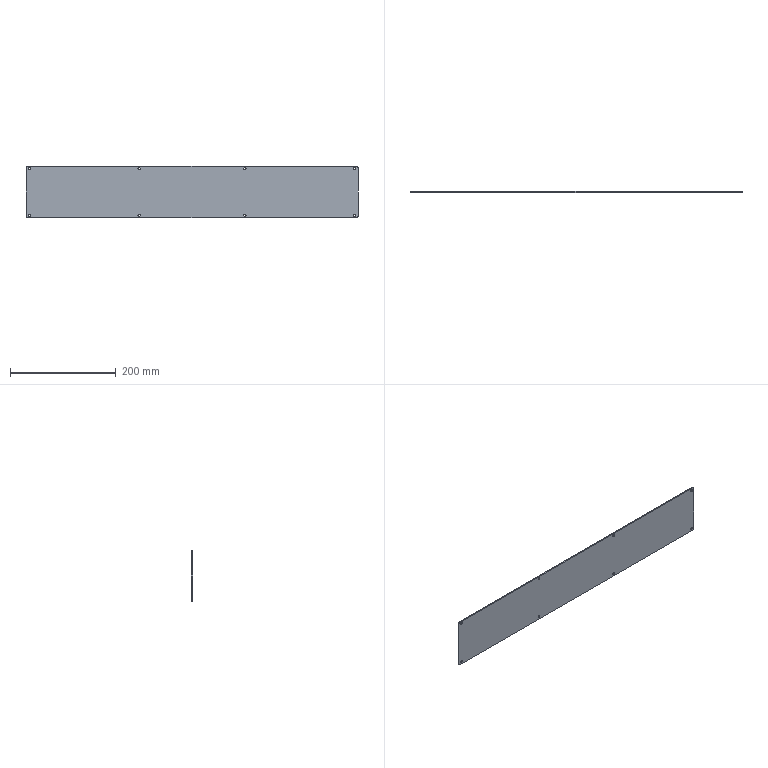Part | SolidWorks | features BaseBody 1 | 1 solid | 26 faces | box 628 x 2 x 98 mm | volume 122818 mm3 | cylinder 20 | plane 6 | commonest cylinder face diameters 4.5 x16 6 x4
STEP:
#1=CARTESIAN_POINT('',(307.5,0.,41.75));
#2=VERTEX_POINT('',#1);
#3=CARTESIAN_POINT('',(307.5,2.,41.75));
#4=VERTEX_POINT('',#3);
#5=CARTESIAN_POINT('',(307.5,-0.001,41.75));
#6=DIRECTION('',(0.,1.,0.));
#7=VECTOR('',#6,1000.);
#8=LINE('',#5,#7);
#9=EDGE_CURVE('',#2,#4,#8,.T.);
#10=ORIENTED_EDGE('',*,*,#9,.F.);
#11=CARTESIAN_POINT('',(307.5,0.,46.25));
#12=VERTEX_POINT('',#11);
#13=CARTESIAN_POINT('',(307.5,0.,44.));
#14=DIRECTION('',(0.,-1.,0.));
#15=DIRECTION('',(0.,0.,1.));
#16=AXIS2_PLACEMENT_3D('',#13,#14,#15);
#17=CIRCLE('',#16,2.25);
#18=EDGE_CURVE('',#2,#12,#17,.T.);
#19=ORIENTED_EDGE('',*,*,#18,.T.);
#20=CARTESIAN_POINT('',(307.5,2.,46.25));
#21=VERTEX_POINT('',#20);
#22=CARTESIAN_POINT('',(307.5,-0.001,46.25));
#23=DIRECTION('',(0.,1.,0.));
#24=VECTOR('',#23,1000.);
#25=LINE('',#22,#24);
#26=EDGE_CURVE('',#12,#21,#25,.T.);
#27=ORIENTED_EDGE('',*,*,#26,.T.);
#28=CARTESIAN_POINT('',(307.5,2.,44.));
#29=DIRECTION('',(0.,1.,0.));
#30=DIRECTION('',(0.,0.,1.));
#31=AXIS2_PLACEMENT_3D('',#28,#29,#30);
#32=CIRCLE('',#31,2.25);
#33=EDGE_CURVE('',#21,#4,#32,.T.);
#34=ORIENTED_EDGE('',*,*,#33,.T.);
#35=EDGE_LOOP('',(#10,#19,#27,#34));
#36=FACE_OUTER_BOUND('',#35,.T.);
#37=CARTESIAN_POINT('',(307.5,-0.001,44.));
#38=DIRECTION('',(0.,1.,0.));
#39=DIRECTION('',(0.,0.,1.));
#40=AXIS2_PLACEMENT_3D('',#37,#38,#39);
#41=CYLINDRICAL_SURFACE('',#40,2.25);
#42=ADVANCED_FACE('',(#36),#41,.F.);
#43=CARTESIAN_POINT('',(-307.5,0.,41.75));
#44=VERTEX_POINT('',#43);
#45=CARTESIAN_POINT('',(-307.5,2.,41.75));
#46=VERTEX_POINT('',#45);
#47=CARTESIAN_POINT('',(-307.5,-0.001,41.75));
#48=DIRECTION('',(0.,1.,0.));
#49=VECTOR('',#48,1000.);
#50=LINE('',#47,#49);
#51=EDGE_CURVE('',#44,#46,#50,.T.);
#52=ORIENTED_EDGE('',*,*,#51,.F.);
#53=CARTESIAN_POINT('',(-307.5,0.,46.25));
#54=VERTEX_POINT('',#53);
#55=CARTESIAN_POINT('',(-307.5,0.,44.));
#56=DIRECTION('',(0.,-1.,0.));
#57=DIRECTION('',(0.,0.,1.));
#58=AXIS2_PLACEMENT_3D('',#55,#56,#57);
#59=CIRCLE('',#58,2.25);
#60=EDGE_CURVE('',#44,#54,#59,.T.);
#61=ORIENTED_EDGE('',*,*,#60,.T.);
#62=CARTESIAN_POINT('',(-307.5,2.,46.25));
#63=VERTEX_POINT('',#62);
#64=CARTESIAN_POINT('',(-307.5,-0.001,46.25));
#65=DIRECTION('',(0.,1.,0.));
#66=VECTOR('',#65,1000.);
#67=LINE('',#64,#66);
#68=EDGE_CURVE('',#54,#63,#67,.T.);
#69=ORIENTED_EDGE('',*,*,#68,.T.);
#70=CARTESIAN_POINT('',(-307.5,2.,44.));
#71=DIRECTION('',(0.,1.,0.));
#72=DIRECTION('',(0.,0.,-1.));
#73=AXIS2_PLACEMENT_3D('',#70,#71,#72);
#74=CIRCLE('',#73,2.25);
#75=EDGE_CURVE('',#63,#46,#74,.T.);
#76=ORIENTED_EDGE('',*,*,#75,.T.);
#77=EDGE_LOOP('',(#52,#61,#69,#76));
#78=FACE_OUTER_BOUND('',#77,.T.);
#79=CARTESIAN_POINT('',(-307.5,-0.001,44.));
#80=DIRECTION('',(0.,1.,0.));
#81=DIRECTION('',(0.,0.,1.));
#82=AXIS2_PLACEMENT_3D('',#79,#80,#81);
#83=CYLINDRICAL_SURFACE('',#82,2.25);
#84=ADVANCED_FACE('',(#78),#83,.F.);
#85=CARTESIAN_POINT('',(-100.,0.,41.75));
#86=VERTEX_POINT('',#85);
#87=CARTESIAN_POINT('',(-100.,2.,41.75));
#88=VERTEX_POINT('',#87);
#89=CARTESIAN_POINT('',(-100.,-0.001,41.75));
#90=DIRECTION('',(0.,1.,0.));
#91=VECTOR('',#90,1000.);
#92=LINE('',#89,#91);
#93=EDGE_CURVE('',#86,#88,#92,.T.);
#94=ORIENTED_EDGE('',*,*,#93,.F.);
#95=CARTESIAN_POINT('',(-100.,0.,46.25));
#96=VERTEX_POINT('',#95);
#97=CARTESIAN_POINT('',(-100.,0.,44.));
#98=DIRECTION('',(0.,-1.,0.));
#99=DIRECTION('',(0.,0.,1.));
#100=AXIS2_PLACEMENT_3D('',#97,#98,#99);
#101=CIRCLE('',#100,2.25);
#102=EDGE_CURVE('',#86,#96,#101,.T.);
#103=ORIENTED_EDGE('',*,*,#102,.T.);
#104=CARTESIAN_POINT('',(-100.,2.,46.25));
#105=VERTEX_POINT('',#104);
#106=CARTESIAN_POINT('',(-100.,-0.001,46.25));
#107=DIRECTION('',(0.,1.,0.));
#108=VECTOR('',#107,1000.);
#109=LINE('',#106,#108);
#110=EDGE_CURVE('',#96,#105,#109,.T.);
#111=ORIENTED_EDGE('',*,*,#110,.T.);
#112=CARTESIAN_POINT('',(-100.,2.,44.));
#113=DIRECTION('',(0.,1.,0.));
#114=DIRECTION('',(0.,0.,-1.));
#115=AXIS2_PLACEMENT_3D('',#112,#113,#114);
#116=CIRCLE('',#115,2.25);
#117=EDGE_CURVE('',#105,#88,#116,.T.);
#118=ORIENTED_EDGE('',*,*,#117,.T.);
#119=EDGE_LOOP('',(#94,#103,#111,#118));
#120=FACE_OUTER_BOUND('',#119,.T.);
#121=CARTESIAN_POINT('',(-100.,-0.001,44.));
#122=DIRECTION('',(0.,1.,0.));
#123=DIRECTION('',(0.,0.,1.));
#124=AXIS2_PLACEMENT_3D('',#121,#122,#123);
#125=CYLINDRICAL_SURFACE('',#124,2.25);
#126=ADVANCED_FACE('',(#120),#125,.F.);
#127=CARTESIAN_POINT('',(-100.,0.,-46.25));
#128=VERTEX_POINT('',#127);
#129=CARTESIAN_POINT('',(-100.,2.,-46.25));
#130=VERTEX_POINT('',#129);
#131=CARTESIAN_POINT('',(-100.,-0.001,-46.25));
#132=DIRECTION('',(0.,1.,0.));
#133=VECTOR('',#132,1000.);
#134=LINE('',#131,#133);
#135=EDGE_CURVE('',#128,#130,#134,.T.);
#136=ORIENTED_EDGE('',*,*,#135,.F.);
#137=CARTESIAN_POINT('',(-100.,0.,-41.75));
#138=VERTEX_POINT('',#137);
#139=CARTESIAN_POINT('',(-100.,0.,-44.));
#140=DIRECTION('',(0.,-1.,0.));
#141=DIRECTION('',(0.,0.,1.));
#142=AXIS2_PLACEMENT_3D('',#139,#140,#141);
#143=CIRCLE('',#142,2.25);
#144=EDGE_CURVE('',#128,#138,#143,.T.);
#145=ORIENTED_EDGE('',*,*,#144,.T.);
#146=CARTESIAN_POINT('',(-100.,2.,-41.75));
#147=VERTEX_POINT('',#146);
#148=CARTESIAN_POINT('',(-100.,-0.001,-41.75));
#149=DIRECTION('',(0.,1.,0.));
#150=VECTOR('',#149,1000.);
#151=LINE('',#148,#150);
#152=EDGE_CURVE('',#138,#147,#151,.T.);
#153=ORIENTED_EDGE('',*,*,#152,.T.);
#154=CARTESIAN_POINT('',(-100.,2.,-44.));
#155=DIRECTION('',(0.,1.,0.));
#156=DIRECTION('',(0.,0.,1.));
#157=AXIS2_PLACEMENT_3D('',#154,#155,#156);
#158=CIRCLE('',#157,2.25);
#159=EDGE_CURVE('',#147,#130,#158,.T.);
#160=ORIENTED_EDGE('',*,*,#159,.T.);
#161=EDGE_LOOP('',(#136,#145,#153,#160));
#162=FACE_OUTER_BOUND('',#161,.T.);
#163=CARTESIAN_POINT('',(-100.,-0.001,-44.));
#164=DIRECTION('',(0.,1.,0.));
#165=DIRECTION('',(0.,0.,1.));
#166=AXIS2_PLACEMENT_3D('',#163,#164,#165);
#167=CYLINDRICAL_SURFACE('',#166,2.25);
#168=ADVANCED_FACE('',(#162),#167,.F.);
#169=CARTESIAN_POINT('',(100.,0.,41.75));
#170=VERTEX_POINT('',#169);
#171=CARTESIAN_POINT('',(100.,2.,41.75));
#172=VERTEX_POINT('',#171);
#173=CARTESIAN_POINT('',(100.,-0.001,41.75));
#174=DIRECTION('',(0.,1.,0.));
#175=VECTOR('',#174,1000.);
#176=LINE('',#173,#175);
#177=EDGE_CURVE('',#170,#172,#176,.T.);
#178=ORIENTED_EDGE('',*,*,#177,.F.);
#179=CARTESIAN_POINT('',(100.,0.,46.25));
#180=VERTEX_POINT('',#179);
#181=CARTESIAN_POINT('',(100.,0.,44.));
#182=DIRECTION('',(0.,-1.,0.));
#183=DIRECTION('',(0.,0.,1.));
#184=AXIS2_PLACEMENT_3D('',#181,#182,#183);
#185=CIRCLE('',#184,2.25);
#186=EDGE_CURVE('',#170,#180,#185,.T.);
#187=ORIENTED_EDGE('',*,*,#186,.T.);
#188=CARTESIAN_POINT('',(100.,2.,46.25));
#189=VERTEX_POINT('',#188);
#190=CARTESIAN_POINT('',(100.,-0.001,46.25));
#191=DIRECTION('',(0.,1.,0.));
#192=VECTOR('',#191,1000.);
#193=LINE('',#190,#192);
#194=EDGE_CURVE('',#180,#189,#193,.T.);
#195=ORIENTED_EDGE('',*,*,#194,.T.);
#196=CARTESIAN_POINT('',(100.,2.,44.));
#197=DIRECTION('',(0.,1.,0.));
#198=DIRECTION('',(0.,0.,1.));
#199=AXIS2_PLACEMENT_3D('',#196,#197,#198);
#200=CIRCLE('',#199,2.25);
#201=EDGE_CURVE('',#189,#172,#200,.T.);
#202=ORIENTED_EDGE('',*,*,#201,.T.);
#203=EDGE_LOOP('',(#178,#187,#195,#202));
#204=FACE_OUTER_BOUND('',#203,.T.);
#205=CARTESIAN_POINT('',(100.,-0.001,44.));
#206=DIRECTION('',(0.,1.,0.));
#207=DIRECTION('',(0.,0.,1.));
#208=AXIS2_PLACEMENT_3D('',#205,#206,#207);
#209=CYLINDRICAL_SURFACE('',#208,2.25);
#210=ADVANCED_FACE('',(#204),#209,.F.);
#211=CARTESIAN_POINT('',(100.,0.,-46.25));
#212=VERTEX_POINT('',#211);
#213=CARTESIAN_POINT('',(100.,2.,-46.25));
#214=VERTEX_POINT('',#213);
#215=CARTESIAN_POINT('',(100.,-0.001,-46.25));
#216=DIRECTION('',(0.,1.,0.));
#217=VECTOR('',#216,1000.);
#218=LINE('',#215,#217);
#219=EDGE_CURVE('',#212,#214,#218,.T.);
#220=ORIENTED_EDGE('',*,*,#219,.F.);
#221=CARTESIAN_POINT('',(100.,0.,-41.75));
#222=VERTEX_POINT('',#221);
#223=CARTESIAN_POINT('',(100.,0.,-44.));
#224=DIRECTION('',(0.,-1.,0.));
#225=DIRECTION('',(0.,0.,1.));
#226=AXIS2_PLACEMENT_3D('',#223,#224,#225);
#227=CIRCLE('',#226,2.25);
#228=EDGE_CURVE('',#212,#222,#227,.T.);
#229=ORIENTED_EDGE('',*,*,#228,.T.);
#230=CARTESIAN_POINT('',(100.,2.,-41.75));
#231=VERTEX_POINT('',#230);
#232=CARTESIAN_POINT('',(100.,-0.001,-41.75));
#233=DIRECTION('',(0.,1.,0.));
#234=VECTOR('',#233,1000.);
#235=LINE('',#232,#234);
#236=EDGE_CURVE('',#222,#231,#235,.T.);
#237=ORIENTED_EDGE('',*,*,#236,.T.);
#238=CARTESIAN_POINT('',(100.,2.,-44.));
#239=DIRECTION('',(0.,1.,0.));
#240=DIRECTION('',(0.,0.,-1.));
#241=AXIS2_PLACEMENT_3D('',#238,#239,#240);
#242=CIRCLE('',#241,2.25);
#243=EDGE_CURVE('',#231,#214,#242,.T.);
#244=ORIENTED_EDGE('',*,*,#243,.T.);
#245=EDGE_LOOP('',(#220,#229,#237,#244));
#246=FACE_OUTER_BOUND('',#245,.T.);
#247=CARTESIAN_POINT('',(100.,-0.001,-44.));
#248=DIRECTION('',(0.,1.,0.));
#249=DIRECTION('',(0.,0.,1.));
#250=AXIS2_PLACEMENT_3D('',#247,#248,#249);
#251=CYLINDRICAL_SURFACE('',#250,2.25);
#252=ADVANCED_FACE('',(#246),#251,.F.);
#253=CARTESIAN_POINT('',(307.5,0.,-46.25));
#254=VERTEX_POINT('',#253);
#255=CARTESIAN_POINT('',(307.5,2.,-46.25));
#256=VERTEX_POINT('',#255);
#257=CARTESIAN_POINT('',(307.5,-0.001,-46.25));
#258=DIRECTION('',(0.,1.,0.));
#259=VECTOR('',#258,1000.);
#260=LINE('',#257,#259);
#261=EDGE_CURVE('',#254,#256,#260,.T.);
#262=ORIENTED_EDGE('',*,*,#261,.F.);
#263=CARTESIAN_POINT('',(307.5,0.,-41.75));
#264=VERTEX_POINT('',#263);
#265=CARTESIAN_POINT('',(307.5,0.,-44.));
#266=DIRECTION('',(0.,-1.,0.));
#267=DIRECTION('',(0.,0.,1.));
#268=AXIS2_PLACEMENT_3D('',#265,#266,#267);
#269=CIRCLE('',#268,2.25);
#270=EDGE_CURVE('',#254,#264,#269,.T.);
#271=ORIENTED_EDGE('',*,*,#270,.T.);
#272=CARTESIAN_POINT('',(307.5,2.,-41.75));
#273=VERTEX_POINT('',#272);
#274=CARTESIAN_POINT('',(307.5,-0.001,-41.75));
#275=DIRECTION('',(0.,1.,0.));
#276=VECTOR('',#275,1000.);
#277=LINE('',#274,#276);
#278=EDGE_CURVE('',#264,#273,#277,.T.);
#279=ORIENTED_EDGE('',*,*,#278,.T.);
#280=CARTESIAN_POINT('',(307.5,2.,-44.));
#281=DIRECTION('',(0.,1.,0.));
#282=DIRECTION('',(0.,0.,-1.));
#283=AXIS2_PLACEMENT_3D('',#280,#281,#282);
#284=CIRCLE('',#283,2.25);
#285=EDGE_CURVE('',#273,#256,#284,.T.);
#286=ORIENTED_EDGE('',*,*,#285,.T.);
#287=EDGE_LOOP('',(#262,#271,#279,#286));
#288=FACE_OUTER_BOUND('',#287,.T.);
#289=CARTESIAN_POINT('',(307.5,-0.001,-44.));
#290=DIRECTION('',(0.,1.,0.));
#291=DIRECTION('',(0.,0.,1.));
#292=AXIS2_PLACEMENT_3D('',#289,#290,#291);
#293=CYLINDRICAL_SURFACE('',#292,2.25);
#294=ADVANCED_FACE('',(#288),#293,.F.);
#295=CARTESIAN_POINT('',(-307.5,0.,-46.25));
#296=VERTEX_POINT('',#295);
#297=CARTESIAN_POINT('',(-307.5,2.,-46.25));
#298=VERTEX_POINT('',#297);
#299=CARTESIAN_POINT('',(-307.5,-0.001,-46.25));
#300=DIRECTION('',(0.,1.,0.));
#301=VECTOR('',#300,1000.);
#302=LINE('',#299,#301);
#303=EDGE_CURVE('',#296,#298,#302,.T.);
#304=ORIENTED_EDGE('',*,*,#303,.F.);
#305=CARTESIAN_POINT('',(-307.5,0.,-41.75));
#306=VERTEX_POINT('',#305);
#307=CARTESIAN_POINT('',(-307.5,0.,-44.));
#308=DIRECTION('',(0.,-1.,0.));
#309=DIRECTION('',(0.,0.,1.));
#310=AXIS2_PLACEMENT_3D('',#307,#308,#309);
#311=CIRCLE('',#310,2.25);
#312=EDGE_CURVE('',#296,#306,#311,.T.);
#313=ORIENTED_EDGE('',*,*,#312,.T.);
#314=CARTESIAN_POINT('',(-307.5,2.,-41.75));
#315=VERTEX_POINT('',#314);
#316=CARTESIAN_POINT('',(-307.5,-0.001,-41.75));
#317=DIRECTION('',(0.,1.,0.));
#318=VECTOR('',#317,1000.);
#319=LINE('',#316,#318);
#320=EDGE_CURVE('',#306,#315,#319,.T.);
#321=ORIENTED_EDGE('',*,*,#320,.T.);
#322=CARTESIAN_POINT('',(-307.5,2.,-44.));
#323=DIRECTION('',(0.,1.,0.));
#324=DIRECTION('',(0.,0.,1.));
#325=AXIS2_PLACEMENT_3D('',#322,#323,#324);
#326=CIRCLE('',#325,2.25);
#327=EDGE_CURVE('',#315,#298,#326,.T.);
#328=ORIENTED_EDGE('',*,*,#327,.T.);
#329=EDGE_LOOP('',(#304,#313,#321,#328));
#330=FACE_OUTER_BOUND('',#329,.T.);
#331=CARTESIAN_POINT('',(-307.5,-0.001,-44.));
#332=DIRECTION('',(0.,1.,0.));
#333=DIRECTION('',(0.,0.,1.));
#334=AXIS2_PLACEMENT_3D('',#331,#332,#333);
#335=CYLINDRICAL_SURFACE('',#334,2.25);
#336=ADVANCED_FACE('',(#330),#335,.F.);
#337=CARTESIAN_POINT('',(311.,2.,49.));
#338=VERTEX_POINT('',#337);
#339=CARTESIAN_POINT('',(314.,2.,46.));
#340=VERTEX_POINT('',#339);
#341=CARTESIAN_POINT('',(311.,2.,46.));
#342=DIRECTION('',(0.,1.,0.));
#343=DIRECTION('',(0.,0.,1.));
#344=AXIS2_PLACEMENT_3D('',#341,#342,#343);
#345=CIRCLE('',#344,3.);
#346=EDGE_CURVE('',#338,#340,#345,.T.);
#347=ORIENTED_EDGE('',*,*,#346,.F.);
#348=CARTESIAN_POINT('',(311.,0.,49.));
#349=VERTEX_POINT('',#348);
#350=CARTESIAN_POINT('',(311.,2.,49.));
#351=DIRECTION('',(0.,1.,0.));
#352=VECTOR('',#351,1000.);
#353=LINE('',#350,#352);
#354=EDGE_CURVE('',#349,#338,#353,.T.);
#355=ORIENTED_EDGE('',*,*,#354,.F.);
#356=CARTESIAN_POINT('',(314.,0.,46.));
#357=VERTEX_POINT('',#356);
#358=CARTESIAN_POINT('',(311.,0.,46.));
#359=DIRECTION('',(0.,-1.,0.));
#360=DIRECTION('',(0.,0.,1.));
#361=AXIS2_PLACEMENT_3D('',#358,#359,#360);
#362=CIRCLE('',#361,3.);
#363=EDGE_CURVE('',#357,#349,#362,.T.);
#364=ORIENTED_EDGE('',*,*,#363,.F.);
#365=CARTESIAN_POINT('',(314.,2.,46.));
#366=DIRECTION('',(0.,-1.,0.));
#367=VECTOR('',#366,1000.);
#368=LINE('',#365,#367);
#369=EDGE_CURVE('',#340,#357,#368,.T.);
#370=ORIENTED_EDGE('',*,*,#369,.F.);
#371=EDGE_LOOP('',(#347,#355,#364,#370));
#372=FACE_OUTER_BOUND('',#371,.T.);
#373=CARTESIAN_POINT('',(311.,2.,46.));
#374=DIRECTION('',(0.,-1.,0.));
#375=DIRECTION('',(0.,0.,-1.));
#376=AXIS2_PLACEMENT_3D('',#373,#374,#375);
#377=CYLINDRICAL_SURFACE('',#376,3.);
#378=ADVANCED_FACE('',(#372),#377,.T.);
#379=CARTESIAN_POINT('',(-314.,2.,46.));
#380=VERTEX_POINT('',#379);
#381=CARTESIAN_POINT('',(-311.,2.,49.));
#382=VERTEX_POINT('',#381);
#383=CARTESIAN_POINT('',(-311.,2.,46.));
#384=DIRECTION('',(0.,1.,0.));
#385=DIRECTION('',(0.,0.,1.));
#386=AXIS2_PLACEMENT_3D('',#383,#384,#385);
#387=CIRCLE('',#386,3.);
#388=EDGE_CURVE('',#380,#382,#387,.T.);
#389=ORIENTED_EDGE('',*,*,#388,.F.);
#390=CARTESIAN_POINT('',(-314.,0.,46.));
#391=VERTEX_POINT('',#390);
#392=CARTESIAN_POINT('',(-314.,2.,46.));
#393=DIRECTION('',(0.,1.,0.));
#394=VECTOR('',#393,1000.);
#395=LINE('',#392,#394);
#396=EDGE_CURVE('',#391,#380,#395,.T.);
#397=ORIENTED_EDGE('',*,*,#396,.F.);
#398=CARTESIAN_POINT('',(-311.,0.,49.));
#399=VERTEX_POINT('',#398);
#400=CARTESIAN_POINT('',(-311.,0.,46.));
#401=DIRECTION('',(0.,-1.,0.));
#402=DIRECTION('',(0.,0.,1.));
#403=AXIS2_PLACEMENT_3D('',#400,#401,#402);
#404=CIRCLE('',#403,3.);
#405=EDGE_CURVE('',#399,#391,#404,.T.);
#406=ORIENTED_EDGE('',*,*,#405,.F.);
#407=CARTESIAN_POINT('',(-311.,2.,49.));
#408=DIRECTION('',(0.,-1.,0.));
#409=VECTOR('',#408,1000.);
#410=LINE('',#407,#409);
#411=EDGE_CURVE('',#382,#399,#410,.T.);
#412=ORIENTED_EDGE('',*,*,#411,.F.);
#413=EDGE_LOOP('',(#389,#397,#406,#412));
#414=FACE_OUTER_BOUND('',#413,.T.);
#415=CARTESIAN_POINT('',(-311.,2.,46.));
#416=DIRECTION('',(0.,-1.,0.));
#417=DIRECTION('',(0.,0.,-1.));
#418=AXIS2_PLACEMENT_3D('',#415,#416,#417);
#419=CYLINDRICAL_SURFACE('',#418,3.);
#420=ADVANCED_FACE('',(#414),#419,.T.);
#421=CARTESIAN_POINT('',(314.,2.,-46.));
#422=VERTEX_POINT('',#421);
#423=CARTESIAN_POINT('',(311.,2.,-49.));
#424=VERTEX_POINT('',#423);
#425=CARTESIAN_POINT('',(311.,2.,-46.));
#426=DIRECTION('',(0.,1.,0.));
#427=DIRECTION('',(0.,0.,1.));
#428=AXIS2_PLACEMENT_3D('',#425,#426,#427);
#429=CIRCLE('',#428,3.);
#430=EDGE_CURVE('',#422,#424,#429,.T.);
#431=ORIENTED_EDGE('',*,*,#430,.F.);
#432=CARTESIAN_POINT('',(314.,0.,-46.));
#433=VERTEX_POINT('',#432);
#434=CARTESIAN_POINT('',(314.,2.,-46.));
#435=DIRECTION('',(0.,1.,0.));
#436=VECTOR('',#435,1000.);
#437=LINE('',#434,#436);
#438=EDGE_CURVE('',#433,#422,#437,.T.);
#439=ORIENTED_EDGE('',*,*,#438,.F.);
#440=CARTESIAN_POINT('',(311.,0.,-49.));
#441=VERTEX_POINT('',#440);
#442=CARTESIAN_POINT('',(311.,0.,-46.));
#443=DIRECTION('',(0.,-1.,0.));
#444=DIRECTION('',(0.,0.,1.));
#445=AXIS2_PLACEMENT_3D('',#442,#443,#444);
#446=CIRCLE('',#445,3.);
#447=EDGE_CURVE('',#441,#433,#446,.T.);
#448=ORIENTED_EDGE('',*,*,#447,.F.);
#449=CARTESIAN_POINT('',(311.,2.,-49.));
#450=DIRECTION('',(0.,-1.,0.));
#451=VECTOR('',#450,1000.);
#452=LINE('',#449,#451);
#453=EDGE_CURVE('',#424,#441,#452,.T.);
#454=ORIENTED_EDGE('',*,*,#453,.F.);
#455=EDGE_LOOP('',(#431,#439,#448,#454));
#456=FACE_OUTER_BOUND('',#455,.T.);
#457=CARTESIAN_POINT('',(311.,2.,-46.));
#458=DIRECTION('',(0.,-1.,0.));
#459=DIRECTION('',(0.,0.,-1.));
#460=AXIS2_PLACEMENT_3D('',#457,#458,#459);
#461=CYLINDRICAL_SURFACE('',#460,3.);
#462=ADVANCED_FACE('',(#456),#461,.T.);
#463=CARTESIAN_POINT('',(-311.,2.,-49.));
#464=VERTEX_POINT('',#463);
#465=CARTESIAN_POINT('',(-314.,2.,-46.));
#466=VERTEX_POINT('',#465);
#467=CARTESIAN_POINT('',(-311.,2.,-46.));
#468=DIRECTION('',(0.,1.,0.));
#469=DIRECTION('',(0.,0.,1.));
#470=AXIS2_PLACEMENT_3D('',#467,#468,#469);
#471=CIRCLE('',#470,3.);
#472=EDGE_CURVE('',#464,#466,#471,.T.);
#473=ORIENTED_EDGE('',*,*,#472,.F.);
#474=CARTESIAN_POINT('',(-311.,0.,-49.));
#475=VERTEX_POINT('',#474);
#476=CARTESIAN_POINT('',(-311.,2.,-49.));
#477=DIRECTION('',(0.,1.,0.));
#478=VECTOR('',#477,1000.);
#479=LINE('',#476,#478);
#480=EDGE_CURVE('',#475,#464,#479,.T.);
#481=ORIENTED_EDGE('',*,*,#480,.F.);
#482=CARTESIAN_POINT('',(-314.,0.,-46.));
#483=VERTEX_POINT('',#482);
#484=CARTESIAN_POINT('',(-311.,0.,-46.));
#485=DIRECTION('',(0.,-1.,0.));
#486=DIRECTION('',(0.,0.,1.));
#487=AXIS2_PLACEMENT_3D('',#484,#485,#486);
#488=CIRCLE('',#487,3.);
#489=EDGE_CURVE('',#483,#475,#488,.T.);
#490=ORIENTED_EDGE('',*,*,#489,.F.);
#491=CARTESIAN_POINT('',(-314.,2.,-46.));
#492=DIRECTION('',(0.,-1.,0.));
#493=VECTOR('',#492,1000.);
#494=LINE('',#491,#493);
#495=EDGE_CURVE('',#466,#483,#494,.T.);
#496=ORIENTED_EDGE('',*,*,#495,.F.);
#497=EDGE_LOOP('',(#473,#481,#490,#496));
#498=FACE_OUTER_BOUND('',#497,.T.);
#499=CARTESIAN_POINT('',(-311.,2.,-46.));
#500=DIRECTION('',(0.,-1.,0.));
#501=DIRECTION('',(0.,0.,-1.));
#502=AXIS2_PLACEMENT_3D('',#499,#500,#501);
#503=CYLINDRICAL_SURFACE('',#502,3.);
#504=ADVANCED_FACE('',(#498),#503,.T.);
#505=CARTESIAN_POINT('',(-307.5,0.,-44.));
#506=DIRECTION('',(0.,-1.,0.));
#507=DIRECTION('',(0.,0.,1.));
#508=AXIS2_PLACEMENT_3D('',#505,#506,#507);
#509=CIRCLE('',#508,2.25);
#510=EDGE_CURVE('',#306,#296,#509,.T.);
#511=ORIENTED_EDGE('',*,*,#510,.F.);
#512=ORIENTED_EDGE('',*,*,#312,.F.);
#513=EDGE_LOOP('',(#511,#512));
#514=FACE_BOUND('',#513,.T.);
#515=CARTESIAN_POINT('',(307.5,0.,-44.));
#516=DIRECTION('',(0.,-1.,0.));
#517=DIRECTION('',(0.,0.,1.));
#518=AXIS2_PLACEMENT_3D('',#515,#516,#517);
#519=CIRCLE('',#518,2.25);
#520=EDGE_CURVE('',#264,#254,#519,.T.);
#521=ORIENTED_EDGE('',*,*,#520,.F.);
#522=ORIENTED_EDGE('',*,*,#270,.F.);
#523=EDGE_LOOP('',(#521,#522));
#524=FACE_BOUND('',#523,.T.);
#525=CARTESIAN_POINT('',(100.,0.,-44.));
#526=DIRECTION('',(0.,-1.,0.));
#527=DIRECTION('',(0.,0.,1.));
#528=AXIS2_PLACEMENT_3D('',#525,#526,#527);
#529=CIRCLE('',#528,2.25);
#530=EDGE_CURVE('',#222,#212,#529,.T.);
#531=ORIENTED_EDGE('',*,*,#530,.F.);
#532=ORIENTED_EDGE('',*,*,#228,.F.);
#533=EDGE_LOOP('',(#531,#532));
#534=FACE_BOUND('',#533,.T.);
#535=CARTESIAN_POINT('',(100.,0.,44.));
#536=DIRECTION('',(0.,-1.,0.));
#537=DIRECTION('',(0.,0.,1.));
#538=AXIS2_PLACEMENT_3D('',#535,#536,#537);
#539=CIRCLE('',#538,2.25);
#540=EDGE_CURVE('',#180,#170,#539,.T.);
#541=ORIENTED_EDGE('',*,*,#540,.F.);
#542=ORIENTED_EDGE('',*,*,#186,.F.);
#543=EDGE_LOOP('',(#541,#542));
#544=FACE_BOUND('',#543,.T.);
#545=CARTESIAN_POINT('',(-100.,0.,-44.));
#546=DIRECTION('',(0.,-1.,0.));
#547=DIRECTION('',(0.,0.,1.));
#548=AXIS2_PLACEMENT_3D('',#545,#546,#547);
#549=CIRCLE('',#548,2.25);
#550=EDGE_CURVE('',#138,#128,#549,.T.);
#551=ORIENTED_EDGE('',*,*,#550,.F.);
#552=ORIENTED_EDGE('',*,*,#144,.F.);
#553=EDGE_LOOP('',(#551,#552));
#554=FACE_BOUND('',#553,.T.);
#555=CARTESIAN_POINT('',(-100.,0.,44.));
#556=DIRECTION('',(0.,-1.,0.));
#557=DIRECTION('',(0.,0.,1.));
#558=AXIS2_PLACEMENT_3D('',#555,#556,#557);
#559=CIRCLE('',#558,2.25);
#560=EDGE_CURVE('',#96,#86,#559,.T.);
#561=ORIENTED_EDGE('',*,*,#560,.F.);
#562=ORIENTED_EDGE('',*,*,#102,.F.);
#563=EDGE_LOOP('',(#561,#562));
#564=FACE_BOUND('',#563,.T.);
#565=CARTESIAN_POINT('',(-307.5,0.,44.));
#566=DIRECTION('',(0.,-1.,0.));
#567=DIRECTION('',(0.,0.,1.));
#568=AXIS2_PLACEMENT_3D('',#565,#566,#567);
#569=CIRCLE('',#568,2.25);
#570=EDGE_CURVE('',#54,#44,#569,.T.);
#571=ORIENTED_EDGE('',*,*,#570,.F.);
#572=ORIENTED_EDGE('',*,*,#60,.F.);
#573=EDGE_LOOP('',(#571,#572));
#574=FACE_BOUND('',#573,.T.);
#575=CARTESIAN_POINT('',(307.5,0.,44.));
#576=DIRECTION('',(0.,-1.,0.));
#577=DIRECTION('',(0.,0.,1.));
#578=AXIS2_PLACEMENT_3D('',#575,#576,#577);
#579=CIRCLE('',#578,2.25);
#580=EDGE_CURVE('',#12,#2,#579,.T.);
#581=ORIENTED_EDGE('',*,*,#580,.F.);
#582=ORIENTED_EDGE('',*,*,#18,.F.);
#583=EDGE_LOOP('',(#581,#582));
#584=FACE_BOUND('',#583,.T.);
#585=CARTESIAN_POINT('',(-314.,0.,49.));
#586=DIRECTION('',(0.,0.,1.));
#587=VECTOR('',#586,1000.);
#588=LINE('',#585,#587);
#589=EDGE_CURVE('',#483,#391,#588,.T.);
#590=ORIENTED_EDGE('',*,*,#589,.F.);
#591=ORIENTED_EDGE('',*,*,#489,.T.);
#592=CARTESIAN_POINT('',(314.,0.,-49.));
#593=DIRECTION('',(-1.,0.,0.));
#594=VECTOR('',#593,1000.);
#595=LINE('',#592,#594);
#596=EDGE_CURVE('',#441,#475,#595,.T.);
#597=ORIENTED_EDGE('',*,*,#596,.F.);
#598=ORIENTED_EDGE('',*,*,#447,.T.);
#599=CARTESIAN_POINT('',(314.,0.,49.));
#600=DIRECTION('',(0.,0.,-1.));
#601=VECTOR('',#600,1000.);
#602=LINE('',#599,#601);
#603=EDGE_CURVE('',#357,#433,#602,.T.);
#604=ORIENTED_EDGE('',*,*,#603,.F.);
#605=ORIENTED_EDGE('',*,*,#363,.T.);
#606=CARTESIAN_POINT('',(314.,0.,49.));
#607=DIRECTION('',(1.,0.,0.));
#608=VECTOR('',#607,1000.);
#609=LINE('',#606,#608);
#610=EDGE_CURVE('',#399,#349,#609,.T.);
#611=ORIENTED_EDGE('',*,*,#610,.F.);
#612=ORIENTED_EDGE('',*,*,#405,.T.);
#613=EDGE_LOOP('',(#590,#591,#597,#598,#604,#605,#611,#612));
#614=FACE_OUTER_BOUND('',#613,.T.);
#615=CARTESIAN_POINT('',(0.,0.,0.));
#616=DIRECTION('',(0.,1.,0.));
#617=DIRECTION('',(1.,0.,0.));
#618=AXIS2_PLACEMENT_3D('',#615,#616,#617);
#619=PLANE('',#618);
#620=ADVANCED_FACE('',(#514,#524,#534,#544,#554,#564,#574,#584,#614),#619,.F.);
#621=ORIENTED_EDGE('',*,*,#327,.F.);
#622=CARTESIAN_POINT('',(-307.5,2.,-44.));
#623=DIRECTION('',(0.,1.,0.));
#624=DIRECTION('',(0.,0.,1.));
#625=AXIS2_PLACEMENT_3D('',#622,#623,#624);
#626=CIRCLE('',#625,2.25);
#627=EDGE_CURVE('',#298,#315,#626,.T.);
#628=ORIENTED_EDGE('',*,*,#627,.F.);
#629=EDGE_LOOP('',(#621,#628));
#630=FACE_BOUND('',#629,.T.);
#631=ORIENTED_EDGE('',*,*,#285,.F.);
#632=CARTESIAN_POINT('',(307.5,2.,-44.));
#633=DIRECTION('',(0.,1.,0.));
#634=DIRECTION('',(0.,0.,-1.));
#635=AXIS2_PLACEMENT_3D('',#632,#633,#634);
#636=CIRCLE('',#635,2.25);
#637=EDGE_CURVE('',#256,#273,#636,.T.);
#638=ORIENTED_EDGE('',*,*,#637,.F.);
#639=EDGE_LOOP('',(#631,#638));
#640=FACE_BOUND('',#639,.T.);
#641=ORIENTED_EDGE('',*,*,#243,.F.);
#642=CARTESIAN_POINT('',(100.,2.,-44.));
#643=DIRECTION('',(0.,1.,0.));
#644=DIRECTION('',(0.,0.,-1.));
#645=AXIS2_PLACEMENT_3D('',#642,#643,#644);
#646=CIRCLE('',#645,2.25);
#647=EDGE_CURVE('',#214,#231,#646,.T.);
#648=ORIENTED_EDGE('',*,*,#647,.F.);
#649=EDGE_LOOP('',(#641,#648));
#650=FACE_BOUND('',#649,.T.);
#651=ORIENTED_EDGE('',*,*,#201,.F.);
#652=CARTESIAN_POINT('',(100.,2.,44.));
#653=DIRECTION('',(0.,1.,0.));
#654=DIRECTION('',(0.,0.,1.));
#655=AXIS2_PLACEMENT_3D('',#652,#653,#654);
#656=CIRCLE('',#655,2.25);
#657=EDGE_CURVE('',#172,#189,#656,.T.);
#658=ORIENTED_EDGE('',*,*,#657,.F.);
#659=EDGE_LOOP('',(#651,#658));
#660=FACE_BOUND('',#659,.T.);
#661=ORIENTED_EDGE('',*,*,#159,.F.);
#662=CARTESIAN_POINT('',(-100.,2.,-44.));
#663=DIRECTION('',(0.,1.,0.));
#664=DIRECTION('',(0.,0.,1.));
#665=AXIS2_PLACEMENT_3D('',#662,#663,#664);
#666=CIRCLE('',#665,2.25);
#667=EDGE_CURVE('',#130,#147,#666,.T.);
#668=ORIENTED_EDGE('',*,*,#667,.F.);
#669=EDGE_LOOP('',(#661,#668));
#670=FACE_BOUND('',#669,.T.);
#671=ORIENTED_EDGE('',*,*,#117,.F.);
#672=CARTESIAN_POINT('',(-100.,2.,44.));
#673=DIRECTION('',(0.,1.,0.));
#674=DIRECTION('',(0.,0.,-1.));
#675=AXIS2_PLACEMENT_3D('',#672,#673,#674);
#676=CIRCLE('',#675,2.25);
#677=EDGE_CURVE('',#88,#105,#676,.T.);
#678=ORIENTED_EDGE('',*,*,#677,.F.);
#679=EDGE_LOOP('',(#671,#678));
#680=FACE_BOUND('',#679,.T.);
#681=ORIENTED_EDGE('',*,*,#75,.F.);
#682=CARTESIAN_POINT('',(-307.5,2.,44.));
#683=DIRECTION('',(0.,1.,0.));
#684=DIRECTION('',(0.,0.,-1.));
#685=AXIS2_PLACEMENT_3D('',#682,#683,#684);
#686=CIRCLE('',#685,2.25);
#687=EDGE_CURVE('',#46,#63,#686,.T.);
#688=ORIENTED_EDGE('',*,*,#687,.F.);
#689=EDGE_LOOP('',(#681,#688));
#690=FACE_BOUND('',#689,.T.);
#691=ORIENTED_EDGE('',*,*,#33,.F.);
#692=CARTESIAN_POINT('',(307.5,2.,44.));
#693=DIRECTION('',(0.,1.,0.));
#694=DIRECTION('',(0.,0.,1.));
#695=AXIS2_PLACEMENT_3D('',#692,#693,#694);
#696=CIRCLE('',#695,2.25);
#697=EDGE_CURVE('',#4,#21,#696,.T.);
#698=ORIENTED_EDGE('',*,*,#697,.F.);
#699=EDGE_LOOP('',(#691,#698));
#700=FACE_BOUND('',#699,.T.);
#701=CARTESIAN_POINT('',(314.,2.,-49.));
#702=DIRECTION('',(-1.,0.,0.));
#703=VECTOR('',#702,1000.);
#704=LINE('',#701,#703);
#705=EDGE_CURVE('',#424,#464,#704,.T.);
#706=ORIENTED_EDGE('',*,*,#705,.T.);
#707=ORIENTED_EDGE('',*,*,#472,.T.);
#708=CARTESIAN_POINT('',(-314.,2.,49.));
#709=DIRECTION('',(0.,0.,1.));
#710=VECTOR('',#709,1000.);
#711=LINE('',#708,#710);
#712=EDGE_CURVE('',#466,#380,#711,.T.);
#713=ORIENTED_EDGE('',*,*,#712,.T.);
#714=ORIENTED_EDGE('',*,*,#388,.T.);
#715=CARTESIAN_POINT('',(314.,2.,49.));
#716=DIRECTION('',(1.,0.,0.));
#717=VECTOR('',#716,1000.);
#718=LINE('',#715,#717);
#719=EDGE_CURVE('',#382,#338,#718,.T.);
#720=ORIENTED_EDGE('',*,*,#719,.T.);
#721=ORIENTED_EDGE('',*,*,#346,.T.);
#722=CARTESIAN_POINT('',(314.,2.,49.));
#723=DIRECTION('',(0.,0.,-1.));
#724=VECTOR('',#723,1000.);
#725=LINE('',#722,#724);
#726=EDGE_CURVE('',#340,#422,#725,.T.);
#727=ORIENTED_EDGE('',*,*,#726,.T.);
#728=ORIENTED_EDGE('',*,*,#430,.T.);
#729=EDGE_LOOP('',(#706,#707,#713,#714,#720,#721,#727,#728));
#730=FACE_OUTER_BOUND('',#729,.T.);
#731=CARTESIAN_POINT('',(0.,2.,0.));
#732=DIRECTION('',(0.,1.,0.));
#733=DIRECTION('',(1.,0.,0.));
#734=AXIS2_PLACEMENT_3D('',#731,#732,#733);
#735=PLANE('',#734);
#736=ADVANCED_FACE('',(#630,#640,#650,#660,#670,#680,#690,#700,#730),#735,.T.);
#737=ORIENTED_EDGE('',*,*,#596,.T.);
#738=ORIENTED_EDGE('',*,*,#480,.T.);
#739=ORIENTED_EDGE('',*,*,#705,.F.);
#740=ORIENTED_EDGE('',*,*,#453,.T.);
#741=EDGE_LOOP('',(#737,#738,#739,#740));
#742=FACE_OUTER_BOUND('',#741,.T.);
#743=CARTESIAN_POINT('',(314.,2.,-49.));
#744=DIRECTION('',(0.,0.,1.));
#745=DIRECTION('',(1.,0.,0.));
#746=AXIS2_PLACEMENT_3D('',#743,#744,#745);
#747=PLANE('',#746);
#748=ADVANCED_FACE('',(#742),#747,.F.);
#749=ORIENTED_EDGE('',*,*,#603,.T.);
#750=ORIENTED_EDGE('',*,*,#438,.T.);
#751=ORIENTED_EDGE('',*,*,#726,.F.);
#752=ORIENTED_EDGE('',*,*,#369,.T.);
#753=EDGE_LOOP('',(#749,#750,#751,#752));
#754=FACE_OUTER_BOUND('',#753,.T.);
#755=CARTESIAN_POINT('',(314.,2.,49.));
#756=DIRECTION('',(-1.,0.,0.));
#757=DIRECTION('',(0.,0.,1.));
#758=AXIS2_PLACEMENT_3D('',#755,#756,#757);
#759=PLANE('',#758);
#760=ADVANCED_FACE('',(#754),#759,.F.);
#761=ORIENTED_EDGE('',*,*,#719,.F.);
#762=ORIENTED_EDGE('',*,*,#411,.T.);
#763=ORIENTED_EDGE('',*,*,#610,.T.);
#764=ORIENTED_EDGE('',*,*,#354,.T.);
#765=EDGE_LOOP('',(#761,#762,#763,#764));
#766=FACE_OUTER_BOUND('',#765,.T.);
#767=CARTESIAN_POINT('',(314.,2.,49.));
#768=DIRECTION('',(0.,0.,-1.));
#769=DIRECTION('',(-1.,0.,0.));
#770=AXIS2_PLACEMENT_3D('',#767,#768,#769);
#771=PLANE('',#770);
#772=ADVANCED_FACE('',(#766),#771,.F.);
#773=ORIENTED_EDGE('',*,*,#712,.F.);
#774=ORIENTED_EDGE('',*,*,#495,.T.);
#775=ORIENTED_EDGE('',*,*,#589,.T.);
#776=ORIENTED_EDGE('',*,*,#396,.T.);
#777=EDGE_LOOP('',(#773,#774,#775,#776));
#778=FACE_OUTER_BOUND('',#777,.T.);
#779=CARTESIAN_POINT('',(-314.,2.,49.));
#780=DIRECTION('',(1.,0.,0.));
#781=DIRECTION('',(0.,1.,0.));
#782=AXIS2_PLACEMENT_3D('',#779,#780,#781);
#783=PLANE('',#782);
#784=ADVANCED_FACE('',(#778),#783,.F.);
#785=ORIENTED_EDGE('',*,*,#510,.T.);
#786=ORIENTED_EDGE('',*,*,#303,.T.);
#787=ORIENTED_EDGE('',*,*,#627,.T.);
#788=ORIENTED_EDGE('',*,*,#320,.F.);
#789=EDGE_LOOP('',(#785,#786,#787,#788));
#790=FACE_OUTER_BOUND('',#789,.T.);
#791=CARTESIAN_POINT('',(-307.5,-0.001,-44.));
#792=DIRECTION('',(0.,1.,0.));
#793=DIRECTION('',(0.,0.,1.));
#794=AXIS2_PLACEMENT_3D('',#791,#792,#793);
#795=CYLINDRICAL_SURFACE('',#794,2.25);
#796=ADVANCED_FACE('',(#790),#795,.F.);
#797=ORIENTED_EDGE('',*,*,#520,.T.);
#798=ORIENTED_EDGE('',*,*,#261,.T.);
#799=ORIENTED_EDGE('',*,*,#637,.T.);
#800=ORIENTED_EDGE('',*,*,#278,.F.);
#801=EDGE_LOOP('',(#797,#798,#799,#800));
#802=FACE_OUTER_BOUND('',#801,.T.);
#803=CARTESIAN_POINT('',(307.5,-0.001,-44.));
#804=DIRECTION('',(0.,1.,0.));
#805=DIRECTION('',(0.,0.,1.));
#806=AXIS2_PLACEMENT_3D('',#803,#804,#805);
#807=CYLINDRICAL_SURFACE('',#806,2.25);
#808=ADVANCED_FACE('',(#802),#807,.F.);
#809=ORIENTED_EDGE('',*,*,#530,.T.);
#810=ORIENTED_EDGE('',*,*,#219,.T.);
#811=ORIENTED_EDGE('',*,*,#647,.T.);
#812=ORIENTED_EDGE('',*,*,#236,.F.);
#813=EDGE_LOOP('',(#809,#810,#811,#812));
#814=FACE_OUTER_BOUND('',#813,.T.);
#815=CARTESIAN_POINT('',(100.,-0.001,-44.));
#816=DIRECTION('',(0.,1.,0.));
#817=DIRECTION('',(0.,0.,1.));
#818=AXIS2_PLACEMENT_3D('',#815,#816,#817);
#819=CYLINDRICAL_SURFACE('',#818,2.25);
#820=ADVANCED_FACE('',(#814),#819,.F.);
#821=ORIENTED_EDGE('',*,*,#540,.T.);
#822=ORIENTED_EDGE('',*,*,#177,.T.);
#823=ORIENTED_EDGE('',*,*,#657,.T.);
#824=ORIENTED_EDGE('',*,*,#194,.F.);
#825=EDGE_LOOP('',(#821,#822,#823,#824));
#826=FACE_OUTER_BOUND('',#825,.T.);
#827=CARTESIAN_POINT('',(100.,-0.001,44.));
#828=DIRECTION('',(0.,1.,0.));
#829=DIRECTION('',(0.,0.,1.));
#830=AXIS2_PLACEMENT_3D('',#827,#828,#829);
#831=CYLINDRICAL_SURFACE('',#830,2.25);
#832=ADVANCED_FACE('',(#826),#831,.F.);
#833=ORIENTED_EDGE('',*,*,#550,.T.);
#834=ORIENTED_EDGE('',*,*,#135,.T.);
#835=ORIENTED_EDGE('',*,*,#667,.T.);
#836=ORIENTED_EDGE('',*,*,#152,.F.);
#837=EDGE_LOOP('',(#833,#834,#835,#836));
#838=FACE_OUTER_BOUND('',#837,.T.);
#839=CARTESIAN_POINT('',(-100.,-0.001,-44.));
#840=DIRECTION('',(0.,1.,0.));
#841=DIRECTION('',(0.,0.,1.));
#842=AXIS2_PLACEMENT_3D('',#839,#840,#841);
#843=CYLINDRICAL_SURFACE('',#842,2.25);
#844=ADVANCED_FACE('',(#838),#843,.F.);
#845=ORIENTED_EDGE('',*,*,#560,.T.);
#846=ORIENTED_EDGE('',*,*,#93,.T.);
#847=ORIENTED_EDGE('',*,*,#677,.T.);
#848=ORIENTED_EDGE('',*,*,#110,.F.);
#849=EDGE_LOOP('',(#845,#846,#847,#848));
#850=FACE_OUTER_BOUND('',#849,.T.);
#851=CARTESIAN_POINT('',(-100.,-0.001,44.));
#852=DIRECTION('',(0.,1.,0.));
#853=DIRECTION('',(0.,0.,1.));
#854=AXIS2_PLACEMENT_3D('',#851,#852,#853);
#855=CYLINDRICAL_SURFACE('',#854,2.25);
#856=ADVANCED_FACE('',(#850),#855,.F.);
#857=ORIENTED_EDGE('',*,*,#570,.T.);
#858=ORIENTED_EDGE('',*,*,#51,.T.);
#859=ORIENTED_EDGE('',*,*,#687,.T.);
#860=ORIENTED_EDGE('',*,*,#68,.F.);
#861=EDGE_LOOP('',(#857,#858,#859,#860));
#862=FACE_OUTER_BOUND('',#861,.T.);
#863=CARTESIAN_POINT('',(-307.5,-0.001,44.));
#864=DIRECTION('',(0.,1.,0.));
#865=DIRECTION('',(0.,0.,1.));
#866=AXIS2_PLACEMENT_3D('',#863,#864,#865);
#867=CYLINDRICAL_SURFACE('',#866,2.25);
#868=ADVANCED_FACE('',(#862),#867,.F.);
#869=ORIENTED_EDGE('',*,*,#580,.T.);
#870=ORIENTED_EDGE('',*,*,#9,.T.);
#871=ORIENTED_EDGE('',*,*,#697,.T.);
#872=ORIENTED_EDGE('',*,*,#26,.F.);
#873=EDGE_LOOP('',(#869,#870,#871,#872));
#874=FACE_OUTER_BOUND('',#873,.T.);
#875=CARTESIAN_POINT('',(307.5,-0.001,44.));
#876=DIRECTION('',(0.,1.,0.));
#877=DIRECTION('',(0.,0.,1.));
#878=AXIS2_PLACEMENT_3D('',#875,#876,#877);
#879=CYLINDRICAL_SURFACE('',#878,2.25);
#880=ADVANCED_FACE('',(#874),#879,.F.);
#881=CLOSED_SHELL('',(#42,#84,#126,#168,#210,#252,#294,#336,#378,#420,#462,#504,#620,#736,#748,#760,#772,#784,#796,#808,#820,#832,#844,#856,#868,#880));
#882=MANIFOLD_SOLID_BREP('',#881);
#883=CARTESIAN_POINT('',(0.,0.,0.));
#884=DIRECTION('',(0.,0.,1.));
#885=DIRECTION('',(1.,0.,0.));
#886=AXIS2_PLACEMENT_3D('',#883,#884,#885);
#887=(LENGTH_UNIT()NAMED_UNIT(*)SI_UNIT(.MILLI.,.METRE.));
#888=UNCERTAINTY_MEASURE_WITH_UNIT(LENGTH_MEASURE(0.00001),#887,'','');
#889=(NAMED_UNIT(*)PLANE_ANGLE_UNIT()SI_UNIT($,.RADIAN.));
#890=(NAMED_UNIT(*)SI_UNIT($,.STERADIAN.)SOLID_ANGLE_UNIT());
#891=(GEOMETRIC_REPRESENTATION_CONTEXT(3)GLOBAL_UNCERTAINTY_ASSIGNED_CONTEXT((#888))GLOBAL_UNIT_ASSIGNED_CONTEXT((#887,#889,#890))REPRESENTATION_CONTEXT('',''));
#892=ADVANCED_BREP_SHAPE_REPRESENTATION('',(#882,#886),#891);